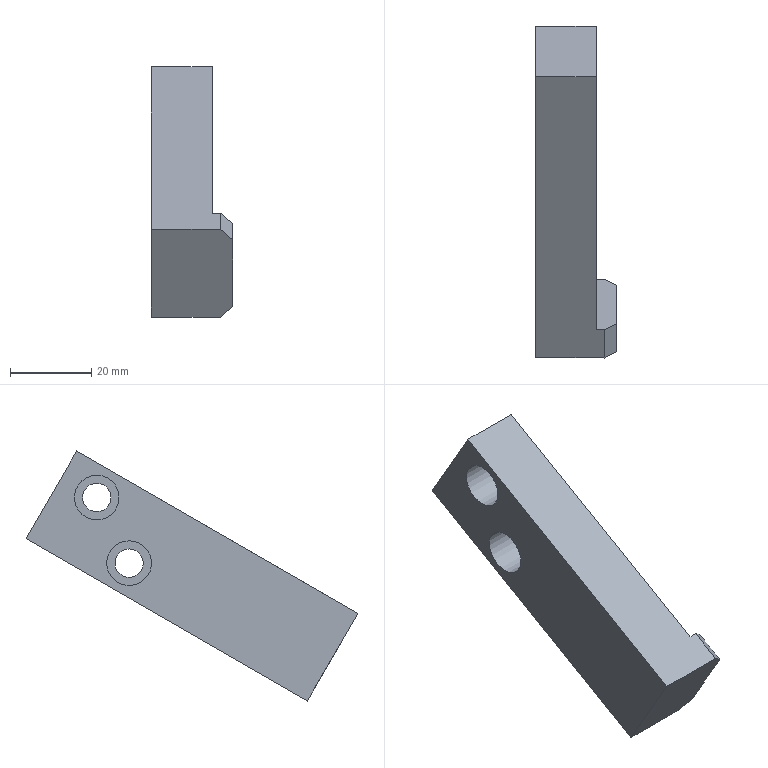Part | NX | features solid 2 | 1 solid | 16 faces | box 20 x 81.782 x 61.652 mm | volume 28752 mm3 | plane 12 | cylinder 4 | commonest cylinder face diameters 7.007 x2 11.008 x2
STEP:
#1=CARTESIAN_POINT('',(-240.023,154.884,54.321));
#2=VERTEX_POINT('',#1);
#3=CARTESIAN_POINT('',(-240.023,154.884,48.817));
#4=DIRECTION('',(1.,0.,-0.000001665));
#5=DIRECTION('',(0.000001665,0.,1.));
#6=AXIS2_PLACEMENT_3D('',#3,#4,#5);
#7=CIRCLE('',#6,5.504);
#8=EDGE_CURVE('',#2,#2,#7,.T.);
#9=ORIENTED_EDGE('',*,*,#8,.T.);
#10=EDGE_LOOP('',(#9));
#11=FACE_BOUND('',#10,.T.);
#12=CARTESIAN_POINT('',(-240.023,180.284,54.822));
#13=VERTEX_POINT('',#12);
#14=CARTESIAN_POINT('',(-240.023,111.003,14.821));
#15=VERTEX_POINT('',#14);
#16=CARTESIAN_POINT('',(-240.023,153.993,39.642));
#17=DIRECTION('',(-0.000000832,-0.866,-0.5));
#18=VECTOR('',#17,1000.);
#19=LINE('',#16,#18);
#20=EDGE_CURVE('',#13,#15,#19,.T.);
#21=ORIENTED_EDGE('',*,*,#20,.T.);
#22=CARTESIAN_POINT('',(-240.023,98.502,36.471));
#23=VERTEX_POINT('',#22);
#24=CARTESIAN_POINT('',(-240.023,105.983,23.514));
#25=DIRECTION('',(-0.000001441,0.5,-0.866));
#26=VECTOR('',#25,1000.);
#27=LINE('',#24,#26);
#28=EDGE_CURVE('',#15,#23,#27,.F.);
#29=ORIENTED_EDGE('',*,*,#28,.T.);
#30=CARTESIAN_POINT('',(-240.023,167.784,76.472));
#31=VERTEX_POINT('',#30);
#32=CARTESIAN_POINT('',(-240.023,167.784,76.472));
#33=DIRECTION('',(0.000000832,0.866,0.5));
#34=VECTOR('',#33,1000.);
#35=LINE('',#32,#34);
#36=EDGE_CURVE('',#23,#31,#35,.T.);
#37=ORIENTED_EDGE('',*,*,#36,.T.);
#38=CARTESIAN_POINT('',(-240.023,175.265,63.515));
#39=DIRECTION('',(0.000001441,-0.5,0.866));
#40=VECTOR('',#39,1000.);
#41=LINE('',#38,#40);
#42=EDGE_CURVE('',#31,#13,#41,.F.);
#43=ORIENTED_EDGE('',*,*,#42,.T.);
#44=EDGE_LOOP('',(#21,#29,#37,#43));
#45=FACE_BOUND('',#44,.T.);
#46=CARTESIAN_POINT('',(-240.023,162.874,70.481));
#47=VERTEX_POINT('',#46);
#48=CARTESIAN_POINT('',(-240.023,162.874,64.977));
#49=DIRECTION('',(1.,0.,-0.000001665));
#50=DIRECTION('',(0.000001665,0.,1.));
#51=AXIS2_PLACEMENT_3D('',#48,#49,#50);
#52=CIRCLE('',#51,5.504);
#53=EDGE_CURVE('',#47,#47,#52,.T.);
#54=ORIENTED_EDGE('',*,*,#53,.T.);
#55=EDGE_LOOP('',(#54));
#56=FACE_BOUND('',#55,.T.);
#57=CARTESIAN_POINT('',(-240.023,175.265,63.515));
#58=DIRECTION('',(-1.,0.,0.000001665));
#59=DIRECTION('',(-0.000001441,0.5,-0.866));
#60=AXIS2_PLACEMENT_3D('',#57,#58,#59);
#61=PLANE('',#60);
#62=ADVANCED_FACE('',(#11,#45,#56),#61,.T.);
#63=CARTESIAN_POINT('',(-223.023,98.502,36.471));
#64=VERTEX_POINT('',#63);
#65=CARTESIAN_POINT('',(-225.023,98.502,36.471));
#66=DIRECTION('',(-1.,0.,0.000001665));
#67=VECTOR('',#66,1000.);
#68=LINE('',#65,#67);
#69=EDGE_CURVE('',#64,#23,#68,.T.);
#70=ORIENTED_EDGE('',*,*,#69,.F.);
#71=CARTESIAN_POINT('',(-223.023,105.43,40.471));
#72=VERTEX_POINT('',#71);
#73=CARTESIAN_POINT('',(-223.023,105.43,40.471));
#74=DIRECTION('',(0.000000832,0.866,0.5));
#75=VECTOR('',#74,1000.);
#76=LINE('',#73,#75);
#77=EDGE_CURVE('',#64,#72,#76,.T.);
#78=ORIENTED_EDGE('',*,*,#77,.T.);
#79=CARTESIAN_POINT('',(-225.023,105.43,40.471));
#80=VERTEX_POINT('',#79);
#81=CARTESIAN_POINT('',(-225.023,105.43,40.471));
#82=DIRECTION('',(1.,0.,-0.000001665));
#83=VECTOR('',#82,1000.);
#84=LINE('',#81,#83);
#85=EDGE_CURVE('',#72,#80,#84,.F.);
#86=ORIENTED_EDGE('',*,*,#85,.T.);
#87=CARTESIAN_POINT('',(-225.023,167.784,76.472));
#88=VERTEX_POINT('',#87);
#89=CARTESIAN_POINT('',(-225.023,167.784,76.472));
#90=DIRECTION('',(0.000000832,0.866,0.5));
#91=VECTOR('',#90,1000.);
#92=LINE('',#89,#91);
#93=EDGE_CURVE('',#80,#88,#92,.T.);
#94=ORIENTED_EDGE('',*,*,#93,.T.);
#95=CARTESIAN_POINT('',(-225.023,167.784,76.472));
#96=DIRECTION('',(1.,0.,-0.000001665));
#97=VECTOR('',#96,1000.);
#98=LINE('',#95,#97);
#99=EDGE_CURVE('',#88,#31,#98,.F.);
#100=ORIENTED_EDGE('',*,*,#99,.T.);
#101=ORIENTED_EDGE('',*,*,#36,.F.);
#102=EDGE_LOOP('',(#70,#78,#86,#94,#100,#101));
#103=FACE_BOUND('',#102,.T.);
#104=CARTESIAN_POINT('',(-225.023,167.784,76.472));
#105=DIRECTION('',(0.000001441,-0.5,0.866));
#106=DIRECTION('',(0.000000832,0.866,0.5));
#107=AXIS2_PLACEMENT_3D('',#104,#105,#106);
#108=PLANE('',#107);
#109=ADVANCED_FACE('',(#103),#108,.T.);
#110=CARTESIAN_POINT('',(-225.023,117.931,18.821));
#111=VERTEX_POINT('',#110);
#112=CARTESIAN_POINT('',(-223.023,117.931,18.821));
#113=VERTEX_POINT('',#112);
#114=CARTESIAN_POINT('',(-225.023,117.931,18.821));
#115=DIRECTION('',(-1.,0.,0.000001665));
#116=VECTOR('',#115,1000.);
#117=LINE('',#114,#116);
#118=EDGE_CURVE('',#111,#113,#117,.F.);
#119=ORIENTED_EDGE('',*,*,#118,.T.);
#120=CARTESIAN_POINT('',(-223.023,111.003,14.821));
#121=VERTEX_POINT('',#120);
#122=CARTESIAN_POINT('',(-223.023,111.003,14.821));
#123=DIRECTION('',(-0.000000832,-0.866,-0.5));
#124=VECTOR('',#123,1000.);
#125=LINE('',#122,#124);
#126=EDGE_CURVE('',#113,#121,#125,.T.);
#127=ORIENTED_EDGE('',*,*,#126,.T.);
#128=CARTESIAN_POINT('',(-225.023,111.003,14.821));
#129=DIRECTION('',(-1.,0.,0.000001665));
#130=VECTOR('',#129,1000.);
#131=LINE('',#128,#130);
#132=EDGE_CURVE('',#121,#15,#131,.T.);
#133=ORIENTED_EDGE('',*,*,#132,.T.);
#134=ORIENTED_EDGE('',*,*,#20,.F.);
#135=CARTESIAN_POINT('',(-225.023,180.284,54.822));
#136=VERTEX_POINT('',#135);
#137=CARTESIAN_POINT('',(-150.099,180.284,54.822));
#138=DIRECTION('',(1.,0.,-0.000001665));
#139=VECTOR('',#138,1000.);
#140=LINE('',#137,#139);
#141=EDGE_CURVE('',#136,#13,#140,.F.);
#142=ORIENTED_EDGE('',*,*,#141,.F.);
#143=CARTESIAN_POINT('',(-225.023,153.993,39.642));
#144=DIRECTION('',(-0.000000832,-0.866,-0.5));
#145=VECTOR('',#144,1000.);
#146=LINE('',#143,#145);
#147=EDGE_CURVE('',#136,#111,#146,.T.);
#148=ORIENTED_EDGE('',*,*,#147,.T.);
#149=EDGE_LOOP('',(#119,#127,#133,#134,#142,#148));
#150=FACE_BOUND('',#149,.T.);
#151=CARTESIAN_POINT('',(-225.023,153.993,39.642));
#152=DIRECTION('',(-0.000001441,0.5,-0.866));
#153=DIRECTION('',(-0.000000832,-0.866,-0.5));
#154=AXIS2_PLACEMENT_3D('',#151,#152,#153);
#155=PLANE('',#154);
#156=ADVANCED_FACE('',(#150),#155,.T.);
#157=CARTESIAN_POINT('',(-225.023,162.874,61.474));
#158=VERTEX_POINT('',#157);
#159=CARTESIAN_POINT('',(-225.023,162.874,64.977));
#160=DIRECTION('',(-1.,0.,0.000001665));
#161=DIRECTION('',(-0.000001665,0.,-1.));
#162=AXIS2_PLACEMENT_3D('',#159,#160,#161);
#163=CIRCLE('',#162,3.503);
#164=EDGE_CURVE('',#158,#158,#163,.T.);
#165=ORIENTED_EDGE('',*,*,#164,.T.);
#166=EDGE_LOOP('',(#165));
#167=FACE_BOUND('',#166,.T.);
#168=CARTESIAN_POINT('',(-225.023,154.884,45.313));
#169=VERTEX_POINT('',#168);
#170=CARTESIAN_POINT('',(-225.023,154.884,48.817));
#171=DIRECTION('',(-1.,0.,0.000001665));
#172=DIRECTION('',(-0.000001665,0.,-1.));
#173=AXIS2_PLACEMENT_3D('',#170,#171,#172);
#174=CIRCLE('',#173,3.503);
#175=EDGE_CURVE('',#169,#169,#174,.T.);
#176=ORIENTED_EDGE('',*,*,#175,.T.);
#177=EDGE_LOOP('',(#176));
#178=FACE_BOUND('',#177,.T.);
#179=CARTESIAN_POINT('',(-225.023,112.911,27.514));
#180=DIRECTION('',(0.000001441,-0.5,0.866));
#181=VECTOR('',#180,1000.);
#182=LINE('',#179,#181);
#183=EDGE_CURVE('',#80,#111,#182,.F.);
#184=ORIENTED_EDGE('',*,*,#183,.T.);
#185=ORIENTED_EDGE('',*,*,#147,.F.);
#186=CARTESIAN_POINT('',(-225.023,175.265,63.515));
#187=DIRECTION('',(0.000001441,-0.5,0.866));
#188=VECTOR('',#187,1000.);
#189=LINE('',#186,#188);
#190=EDGE_CURVE('',#88,#136,#189,.F.);
#191=ORIENTED_EDGE('',*,*,#190,.F.);
#192=ORIENTED_EDGE('',*,*,#93,.F.);
#193=EDGE_LOOP('',(#184,#185,#191,#192));
#194=FACE_BOUND('',#193,.T.);
#195=CARTESIAN_POINT('',(-225.023,175.265,63.515));
#196=DIRECTION('',(-1.,0.,0.000001665));
#197=DIRECTION('',(-0.000001441,0.5,-0.866));
#198=AXIS2_PLACEMENT_3D('',#195,#196,#197);
#199=PLANE('',#198);
#200=ADVANCED_FACE('',(#167,#178,#194),#199,.F.);
#201=ORIENTED_EDGE('',*,*,#99,.F.);
#202=ORIENTED_EDGE('',*,*,#190,.T.);
#203=ORIENTED_EDGE('',*,*,#141,.T.);
#204=ORIENTED_EDGE('',*,*,#42,.F.);
#205=EDGE_LOOP('',(#201,#202,#203,#204));
#206=FACE_BOUND('',#205,.T.);
#207=CARTESIAN_POINT('',(-150.099,185.265,46.195));
#208=DIRECTION('',(-0.000000832,-0.866,-0.5));
#209=DIRECTION('',(0.000001441,-0.5,0.866));
#210=AXIS2_PLACEMENT_3D('',#207,#208,#209);
#211=PLANE('',#210);
#212=ADVANCED_FACE('',(#206),#211,.F.);
#213=ORIENTED_EDGE('',*,*,#132,.F.);
#214=CARTESIAN_POINT('',(-220.023,109.503,17.419));
#215=VERTEX_POINT('',#214);
#216=CARTESIAN_POINT('',(-219.004,108.993,18.301));
#217=DIRECTION('',(0.7071,-0.3536,0.6124));
#218=VECTOR('',#217,1000.);
#219=LINE('',#216,#218);
#220=EDGE_CURVE('',#121,#215,#219,.T.);
#221=ORIENTED_EDGE('',*,*,#220,.T.);
#222=CARTESIAN_POINT('',(-220.023,100.002,33.873));
#223=VERTEX_POINT('',#222);
#224=CARTESIAN_POINT('',(-220.023,105.983,23.514));
#225=DIRECTION('',(0.000001441,-0.5,0.866));
#226=VECTOR('',#225,1000.);
#227=LINE('',#224,#226);
#228=EDGE_CURVE('',#215,#223,#227,.T.);
#229=ORIENTED_EDGE('',*,*,#228,.T.);
#230=CARTESIAN_POINT('',(-216.542,101.743,30.859));
#231=DIRECTION('',(-0.7071,-0.3536,0.6124));
#232=VECTOR('',#231,1000.);
#233=LINE('',#230,#232);
#234=EDGE_CURVE('',#223,#64,#233,.T.);
#235=ORIENTED_EDGE('',*,*,#234,.T.);
#236=ORIENTED_EDGE('',*,*,#69,.T.);
#237=ORIENTED_EDGE('',*,*,#28,.F.);
#238=EDGE_LOOP('',(#213,#221,#229,#235,#236,#237));
#239=FACE_BOUND('',#238,.T.);
#240=CARTESIAN_POINT('',(-225.023,105.983,23.514));
#241=DIRECTION('',(-0.000000832,-0.866,-0.5));
#242=DIRECTION('',(0.000001441,-0.5,0.866));
#243=AXIS2_PLACEMENT_3D('',#240,#241,#242);
#244=PLANE('',#243);
#245=ADVANCED_FACE('',(#239),#244,.T.);
#246=ORIENTED_EDGE('',*,*,#228,.F.);
#247=CARTESIAN_POINT('',(-220.023,116.431,21.419));
#248=VERTEX_POINT('',#247);
#249=CARTESIAN_POINT('',(-220.023,116.431,21.419));
#250=DIRECTION('',(0.000000832,0.866,0.5));
#251=VECTOR('',#250,1000.);
#252=LINE('',#249,#251);
#253=EDGE_CURVE('',#215,#248,#252,.T.);
#254=ORIENTED_EDGE('',*,*,#253,.T.);
#255=CARTESIAN_POINT('',(-220.023,106.93,37.873));
#256=VERTEX_POINT('',#255);
#257=CARTESIAN_POINT('',(-220.023,112.911,27.514));
#258=DIRECTION('',(0.000001441,-0.5,0.866));
#259=VECTOR('',#258,1000.);
#260=LINE('',#257,#259);
#261=EDGE_CURVE('',#248,#256,#260,.T.);
#262=ORIENTED_EDGE('',*,*,#261,.T.);
#263=CARTESIAN_POINT('',(-220.023,100.002,33.873));
#264=DIRECTION('',(-0.000000832,-0.866,-0.5));
#265=VECTOR('',#264,1000.);
#266=LINE('',#263,#265);
#267=EDGE_CURVE('',#256,#223,#266,.T.);
#268=ORIENTED_EDGE('',*,*,#267,.T.);
#269=EDGE_LOOP('',(#246,#254,#262,#268));
#270=FACE_BOUND('',#269,.T.);
#271=CARTESIAN_POINT('',(-220.023,175.265,63.515));
#272=DIRECTION('',(-1.,0.,0.000001665));
#273=DIRECTION('',(-0.000001441,0.5,-0.866));
#274=AXIS2_PLACEMENT_3D('',#271,#272,#273);
#275=PLANE('',#274);
#276=ADVANCED_FACE('',(#270),#275,.F.);
#277=ORIENTED_EDGE('',*,*,#261,.F.);
#278=CARTESIAN_POINT('',(-223.023,117.931,18.821));
#279=DIRECTION('',(-0.7071,0.3536,-0.6124));
#280=VECTOR('',#279,1000.);
#281=LINE('',#278,#280);
#282=EDGE_CURVE('',#248,#113,#281,.T.);
#283=ORIENTED_EDGE('',*,*,#282,.T.);
#284=ORIENTED_EDGE('',*,*,#118,.F.);
#285=ORIENTED_EDGE('',*,*,#183,.F.);
#286=ORIENTED_EDGE('',*,*,#85,.F.);
#287=CARTESIAN_POINT('',(-223.023,105.43,40.471));
#288=DIRECTION('',(0.7071,0.3536,-0.6124));
#289=VECTOR('',#288,1000.);
#290=LINE('',#287,#289);
#291=EDGE_CURVE('',#72,#256,#290,.T.);
#292=ORIENTED_EDGE('',*,*,#291,.T.);
#293=EDGE_LOOP('',(#277,#283,#284,#285,#286,#292));
#294=FACE_BOUND('',#293,.T.);
#295=CARTESIAN_POINT('',(-232.523,111.681,29.646));
#296=DIRECTION('',(-0.000000832,-0.866,-0.5));
#297=DIRECTION('',(0.,-0.5,0.866));
#298=AXIS2_PLACEMENT_3D('',#295,#296,#297);
#299=PLANE('',#298);
#300=ADVANCED_FACE('',(#294),#299,.F.);
#301=ORIENTED_EDGE('',*,*,#282,.F.);
#302=ORIENTED_EDGE('',*,*,#253,.F.);
#303=ORIENTED_EDGE('',*,*,#220,.F.);
#304=ORIENTED_EDGE('',*,*,#126,.F.);
#305=EDGE_LOOP('',(#301,#302,#303,#304));
#306=FACE_BOUND('',#305,.T.);
#307=CARTESIAN_POINT('',(-223.023,153.993,39.642));
#308=DIRECTION('',(0.7071,0.3536,-0.6124));
#309=DIRECTION('',(0.000000832,0.866,0.5));
#310=AXIS2_PLACEMENT_3D('',#307,#308,#309);
#311=PLANE('',#310);
#312=ADVANCED_FACE('',(#306),#311,.T.);
#313=ORIENTED_EDGE('',*,*,#234,.F.);
#314=ORIENTED_EDGE('',*,*,#267,.F.);
#315=ORIENTED_EDGE('',*,*,#291,.F.);
#316=ORIENTED_EDGE('',*,*,#77,.F.);
#317=EDGE_LOOP('',(#313,#314,#315,#316));
#318=FACE_BOUND('',#317,.T.);
#319=CARTESIAN_POINT('',(-223.023,167.784,76.472));
#320=DIRECTION('',(0.7071,-0.3536,0.6124));
#321=DIRECTION('',(-0.000000832,-0.866,-0.5));
#322=AXIS2_PLACEMENT_3D('',#319,#320,#321);
#323=PLANE('',#322);
#324=ADVANCED_FACE('',(#318),#323,.T.);
#325=CARTESIAN_POINT('',(-231.023,154.884,52.32));
#326=VERTEX_POINT('',#325);
#327=CARTESIAN_POINT('',(-231.023,154.884,48.817));
#328=DIRECTION('',(1.,0.,-0.000001665));
#329=DIRECTION('',(0.000001665,0.,1.));
#330=AXIS2_PLACEMENT_3D('',#327,#328,#329);
#331=CIRCLE('',#330,3.503);
#332=EDGE_CURVE('',#326,#326,#331,.T.);
#333=ORIENTED_EDGE('',*,*,#332,.F.);
#334=EDGE_LOOP('',(#333));
#335=FACE_BOUND('',#334,.T.);
#336=ORIENTED_EDGE('',*,*,#175,.F.);
#337=EDGE_LOOP('',(#336));
#338=FACE_BOUND('',#337,.T.);
#339=CARTESIAN_POINT('',(-240.023,154.884,48.817));
#340=DIRECTION('',(1.,0.,-0.000001665));
#341=DIRECTION('',(0.000001665,0.,1.));
#342=AXIS2_PLACEMENT_3D('',#339,#340,#341);
#343=CYLINDRICAL_SURFACE('',#342,3.503);
#344=ADVANCED_FACE('',(#335,#338),#343,.F.);
#345=ORIENTED_EDGE('',*,*,#332,.T.);
#346=EDGE_LOOP('',(#345));
#347=FACE_BOUND('',#346,.T.);
#348=CARTESIAN_POINT('',(-231.023,154.884,54.321));
#349=VERTEX_POINT('',#348);
#350=CARTESIAN_POINT('',(-231.023,154.884,48.817));
#351=DIRECTION('',(-1.,0.,0.000001665));
#352=DIRECTION('',(0.000001665,0.,1.));
#353=AXIS2_PLACEMENT_3D('',#350,#351,#352);
#354=CIRCLE('',#353,5.504);
#355=EDGE_CURVE('',#349,#349,#354,.F.);
#356=ORIENTED_EDGE('',*,*,#355,.F.);
#357=EDGE_LOOP('',(#356));
#358=FACE_BOUND('',#357,.T.);
#359=CARTESIAN_POINT('',(-231.023,154.884,48.817));
#360=DIRECTION('',(1.,0.,-0.000001665));
#361=DIRECTION('',(0.000001665,0.,1.));
#362=AXIS2_PLACEMENT_3D('',#359,#360,#361);
#363=PLANE('',#362);
#364=ADVANCED_FACE('',(#347,#358),#363,.F.);
#365=ORIENTED_EDGE('',*,*,#355,.T.);
#366=EDGE_LOOP('',(#365));
#367=FACE_BOUND('',#366,.T.);
#368=ORIENTED_EDGE('',*,*,#8,.F.);
#369=EDGE_LOOP('',(#368));
#370=FACE_BOUND('',#369,.T.);
#371=CARTESIAN_POINT('',(-240.023,154.884,48.817));
#372=DIRECTION('',(1.,0.,-0.000001665));
#373=DIRECTION('',(0.000001665,0.,1.));
#374=AXIS2_PLACEMENT_3D('',#371,#372,#373);
#375=CYLINDRICAL_SURFACE('',#374,5.504);
#376=ADVANCED_FACE('',(#367,#370),#375,.F.);
#377=CARTESIAN_POINT('',(-231.023,162.874,68.481));
#378=VERTEX_POINT('',#377);
#379=CARTESIAN_POINT('',(-231.023,162.874,64.977));
#380=DIRECTION('',(1.,0.,-0.000001665));
#381=DIRECTION('',(0.000001665,0.,1.));
#382=AXIS2_PLACEMENT_3D('',#379,#380,#381);
#383=CIRCLE('',#382,3.503);
#384=EDGE_CURVE('',#378,#378,#383,.T.);
#385=ORIENTED_EDGE('',*,*,#384,.F.);
#386=EDGE_LOOP('',(#385));
#387=FACE_BOUND('',#386,.T.);
#388=ORIENTED_EDGE('',*,*,#164,.F.);
#389=EDGE_LOOP('',(#388));
#390=FACE_BOUND('',#389,.T.);
#391=CARTESIAN_POINT('',(-240.023,162.874,64.977));
#392=DIRECTION('',(1.,0.,-0.000001665));
#393=DIRECTION('',(0.000001665,0.,1.));
#394=AXIS2_PLACEMENT_3D('',#391,#392,#393);
#395=CYLINDRICAL_SURFACE('',#394,3.503);
#396=ADVANCED_FACE('',(#387,#390),#395,.F.);
#397=ORIENTED_EDGE('',*,*,#384,.T.);
#398=EDGE_LOOP('',(#397));
#399=FACE_BOUND('',#398,.T.);
#400=CARTESIAN_POINT('',(-231.023,162.874,70.481));
#401=VERTEX_POINT('',#400);
#402=CARTESIAN_POINT('',(-231.023,162.874,64.977));
#403=DIRECTION('',(-1.,0.,0.000001665));
#404=DIRECTION('',(0.000001665,0.,1.));
#405=AXIS2_PLACEMENT_3D('',#402,#403,#404);
#406=CIRCLE('',#405,5.504);
#407=EDGE_CURVE('',#401,#401,#406,.F.);
#408=ORIENTED_EDGE('',*,*,#407,.F.);
#409=EDGE_LOOP('',(#408));
#410=FACE_BOUND('',#409,.T.);
#411=CARTESIAN_POINT('',(-231.023,162.874,64.977));
#412=DIRECTION('',(1.,0.,-0.000001665));
#413=DIRECTION('',(0.000001665,0.,1.));
#414=AXIS2_PLACEMENT_3D('',#411,#412,#413);
#415=PLANE('',#414);
#416=ADVANCED_FACE('',(#399,#410),#415,.F.);
#417=ORIENTED_EDGE('',*,*,#407,.T.);
#418=EDGE_LOOP('',(#417));
#419=FACE_BOUND('',#418,.T.);
#420=ORIENTED_EDGE('',*,*,#53,.F.);
#421=EDGE_LOOP('',(#420));
#422=FACE_BOUND('',#421,.T.);
#423=CARTESIAN_POINT('',(-240.023,162.874,64.977));
#424=DIRECTION('',(1.,0.,-0.000001665));
#425=DIRECTION('',(0.000001665,0.,1.));
#426=AXIS2_PLACEMENT_3D('',#423,#424,#425);
#427=CYLINDRICAL_SURFACE('',#426,5.504);
#428=ADVANCED_FACE('',(#419,#422),#427,.F.);
#429=CLOSED_SHELL('',(#62,#109,#156,#200,#212,#245,#276,#300,#312,#324,#344,#364,#376,#396,#416,#428));
#430=MANIFOLD_SOLID_BREP('',#429);
#431=(LENGTH_UNIT()NAMED_UNIT(*)SI_UNIT(.MILLI.,.METRE.));
#432=UNCERTAINTY_MEASURE_WITH_UNIT(LENGTH_MEASURE(0.00001),#431,'','');
#433=(NAMED_UNIT(*)PLANE_ANGLE_UNIT()SI_UNIT($,.RADIAN.));
#434=(NAMED_UNIT(*)SI_UNIT($,.STERADIAN.)SOLID_ANGLE_UNIT());
#435=(GEOMETRIC_REPRESENTATION_CONTEXT(3)GLOBAL_UNCERTAINTY_ASSIGNED_CONTEXT((#432))GLOBAL_UNIT_ASSIGNED_CONTEXT((#431,#433,#434))REPRESENTATION_CONTEXT('',''));
#436=ADVANCED_BREP_SHAPE_REPRESENTATION('',(#430),#435);